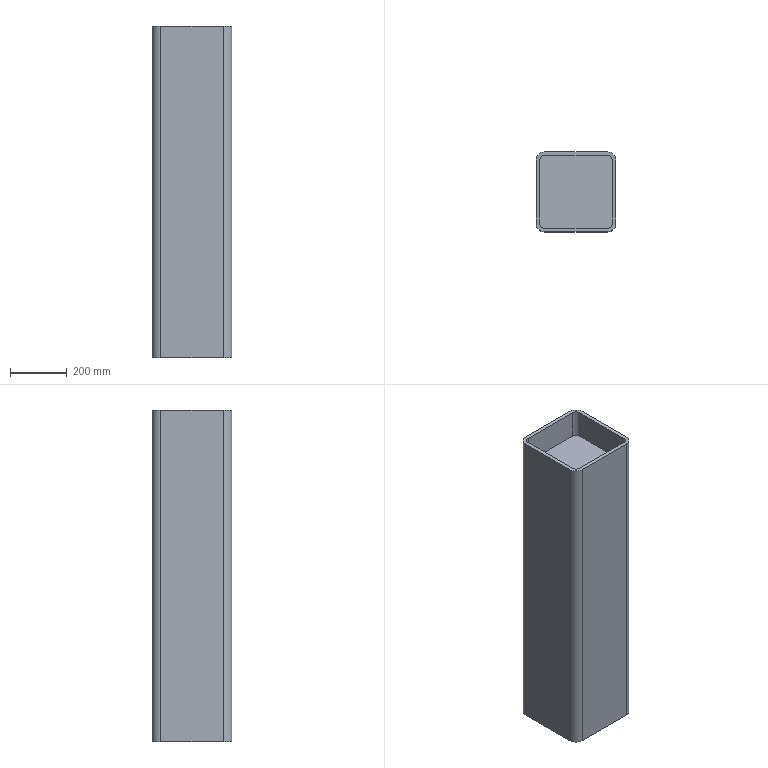Part | SolidWorks | features ICE 2, Extrusion 1, MirrorPattern 1 | 1 solid | 58 faces | box 280 x 280 x 1165 mm | volume 17020849 mm3 | plane 34 | cylinder 24 | commonest cylinder face diameters 36 x20 60 x4